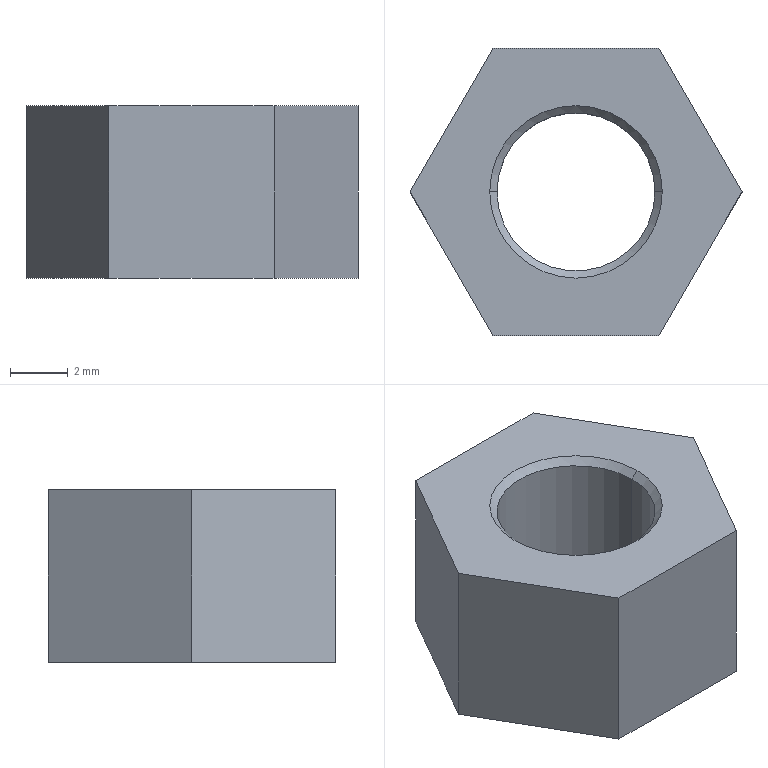Part | STEP file | Tan M6 | 1 solid | 14 faces | box 11.547 x 10 x 6 mm | volume 375.953 mm3 | plane 8 | cone 4 | cylinder 2 | commonest cylinder face diameters 5.5 x2
STEP:
#1=CARTESIAN_POINT('',(0.,0.,0.));
#2=DIRECTION('',(0.,0.,1.));
#3=DIRECTION('',(1.,0.,0.));
#4=AXIS2_PLACEMENT_3D('',#1,#2,#3);
#5=CARTESIAN_POINT('',(-2.75,0.,0.25));
#6=VERTEX_POINT('',#5);
#7=CARTESIAN_POINT('',(-3.,0.,0.));
#8=VERTEX_POINT('',#7);
#9=CARTESIAN_POINT('',(-3.,0.,0.));
#10=DIRECTION('',(-0.7071,0.,-0.7071));
#11=VECTOR('',#10,1.);
#12=LINE('',#9,#11);
#13=CARTESIAN_POINT('',(0.,0.,0.));
#14=DIRECTION('',(0.,0.,-1.));
#15=DIRECTION('',(-1.,0.,0.));
#16=AXIS2_PLACEMENT_3D('',#13,#14,#15);
#17=CONICAL_SURFACE('',#16,3.,0.7854);
#18=CARTESIAN_POINT('',(6.283,0.));
#19=DIRECTION('',(0.,1.));
#20=VECTOR('',#19,1.);
#21=LINE('',#18,#20);
#22=(GEOMETRIC_REPRESENTATION_CONTEXT(2)PARAMETRIC_REPRESENTATION_CONTEXT()REPRESENTATION_CONTEXT('',''));
#23=DEFINITIONAL_REPRESENTATION('',(#21),#22);
#24=PCURVE('',#17,#23);
#25=CARTESIAN_POINT('',(0.,0.,0.));
#26=DIRECTION('',(0.,0.,-1.));
#27=DIRECTION('',(-1.,0.,0.));
#28=AXIS2_PLACEMENT_3D('',#25,#26,#27);
#29=CONICAL_SURFACE('',#28,3.,0.7854);
#30=CARTESIAN_POINT('',(0.,0.));
#31=DIRECTION('',(0.,1.));
#32=VECTOR('',#31,1.);
#33=LINE('',#30,#32);
#34=(GEOMETRIC_REPRESENTATION_CONTEXT(2)PARAMETRIC_REPRESENTATION_CONTEXT()REPRESENTATION_CONTEXT('',''));
#35=DEFINITIONAL_REPRESENTATION('',(#33),#34);
#36=PCURVE('',#29,#35);
#37=SURFACE_CURVE('',#12,(#24,#36),.PCURVE_S1.);
#38=EDGE_CURVE('',#6,#8,#37,.T.);
#39=ORIENTED_EDGE('',*,*,#38,.T.);
#40=CARTESIAN_POINT('',(3.,0.,0.));
#41=VERTEX_POINT('',#40);
#42=CARTESIAN_POINT('',(0.,0.,0.));
#43=DIRECTION('',(0.,0.,1.));
#44=DIRECTION('',(1.,0.,0.));
#45=AXIS2_PLACEMENT_3D('',#42,#43,#44);
#46=CIRCLE('',#45,3.);
#47=CARTESIAN_POINT('',(9.425,0.));
#48=DIRECTION('',(-1.,0.));
#49=VECTOR('',#48,1.);
#50=LINE('',#47,#49);
#51=(GEOMETRIC_REPRESENTATION_CONTEXT(2)PARAMETRIC_REPRESENTATION_CONTEXT()REPRESENTATION_CONTEXT('',''));
#52=DEFINITIONAL_REPRESENTATION('',(#50),#51);
#53=PCURVE('',#17,#52);
#54=CARTESIAN_POINT('',(0.,0.,0.));
#55=DIRECTION('',(0.,0.,1.));
#56=DIRECTION('',(1.,0.,0.));
#57=AXIS2_PLACEMENT_3D('',#54,#55,#56);
#58=PLANE('',#57);
#59=CARTESIAN_POINT('',(0.,0.));
#60=DIRECTION('',(1.,0.));
#61=AXIS2_PLACEMENT_2D('',#59,#60);
#62=CIRCLE('',#61,3.);
#63=(GEOMETRIC_REPRESENTATION_CONTEXT(2)PARAMETRIC_REPRESENTATION_CONTEXT()REPRESENTATION_CONTEXT('',''));
#64=DEFINITIONAL_REPRESENTATION('',(#62),#63);
#65=PCURVE('',#58,#64);
#66=SURFACE_CURVE('',#46,(#53,#65),.PCURVE_S1.);
#67=EDGE_CURVE('',#8,#41,#66,.T.);
#68=ORIENTED_EDGE('',*,*,#67,.T.);
#69=CARTESIAN_POINT('',(2.75,0.,0.25));
#70=VERTEX_POINT('',#69);
#71=CARTESIAN_POINT('',(3.,0.,0.));
#72=DIRECTION('',(0.7071,0.,-0.7071));
#73=VECTOR('',#72,1.);
#74=LINE('',#71,#73);
#75=CARTESIAN_POINT('',(3.142,0.));
#76=DIRECTION('',(0.,1.));
#77=VECTOR('',#76,1.);
#78=LINE('',#75,#77);
#79=(GEOMETRIC_REPRESENTATION_CONTEXT(2)PARAMETRIC_REPRESENTATION_CONTEXT()REPRESENTATION_CONTEXT('',''));
#80=DEFINITIONAL_REPRESENTATION('',(#78),#79);
#81=PCURVE('',#17,#80);
#82=CARTESIAN_POINT('',(3.142,0.));
#83=DIRECTION('',(0.,1.));
#84=VECTOR('',#83,1.);
#85=LINE('',#82,#84);
#86=(GEOMETRIC_REPRESENTATION_CONTEXT(2)PARAMETRIC_REPRESENTATION_CONTEXT()REPRESENTATION_CONTEXT('',''));
#87=DEFINITIONAL_REPRESENTATION('',(#85),#86);
#88=PCURVE('',#29,#87);
#89=SURFACE_CURVE('',#74,(#81,#88),.PCURVE_S1.);
#90=EDGE_CURVE('',#70,#41,#89,.T.);
#91=ORIENTED_EDGE('',*,*,#90,.F.);
#92=CARTESIAN_POINT('',(0.,0.,0.25));
#93=DIRECTION('',(0.,0.,-1.));
#94=DIRECTION('',(1.,0.,0.));
#95=AXIS2_PLACEMENT_3D('',#92,#93,#94);
#96=CIRCLE('',#95,2.75);
#97=CARTESIAN_POINT('',(3.142,-0.25));
#98=DIRECTION('',(1.,0.));
#99=VECTOR('',#98,1.);
#100=LINE('',#97,#99);
#101=(GEOMETRIC_REPRESENTATION_CONTEXT(2)PARAMETRIC_REPRESENTATION_CONTEXT()REPRESENTATION_CONTEXT('',''));
#102=DEFINITIONAL_REPRESENTATION('',(#100),#101);
#103=PCURVE('',#17,#102);
#104=CARTESIAN_POINT('',(0.,0.,6.));
#105=DIRECTION('',(0.,0.,-1.));
#106=DIRECTION('',(-1.,0.,0.));
#107=AXIS2_PLACEMENT_3D('',#104,#105,#106);
#108=CYLINDRICAL_SURFACE('',#107,2.75);
#109=CARTESIAN_POINT('',(3.142,5.75));
#110=DIRECTION('',(1.,0.));
#111=VECTOR('',#110,1.);
#112=LINE('',#109,#111);
#113=(GEOMETRIC_REPRESENTATION_CONTEXT(2)PARAMETRIC_REPRESENTATION_CONTEXT()REPRESENTATION_CONTEXT('',''));
#114=DEFINITIONAL_REPRESENTATION('',(#112),#113);
#115=PCURVE('',#108,#114);
#116=SURFACE_CURVE('',#96,(#103,#115),.PCURVE_S1.);
#117=EDGE_CURVE('',#70,#6,#116,.T.);
#118=ORIENTED_EDGE('',*,*,#117,.T.);
#119=EDGE_LOOP('',(#39,#68,#91,#118));
#120=FACE_BOUND('',#119,.F.);
#121=ADVANCED_FACE('',(#120),#17,.F.);
#122=CARTESIAN_POINT('',(2.75,0.,5.75));
#123=VERTEX_POINT('',#122);
#124=CARTESIAN_POINT('',(3.,0.,6.));
#125=VERTEX_POINT('',#124);
#126=CARTESIAN_POINT('',(2.75,0.,5.75));
#127=DIRECTION('',(0.7071,0.,0.7071));
#128=VECTOR('',#127,1.);
#129=LINE('',#126,#128);
#130=CARTESIAN_POINT('',(0.,0.,5.75));
#131=DIRECTION('',(0.,0.,1.));
#132=DIRECTION('',(1.,0.,0.));
#133=AXIS2_PLACEMENT_3D('',#130,#131,#132);
#134=CONICAL_SURFACE('',#133,2.75,0.7854);
#135=CARTESIAN_POINT('',(6.283,0.));
#136=DIRECTION('',(0.,1.));
#137=VECTOR('',#136,1.);
#138=LINE('',#135,#137);
#139=(GEOMETRIC_REPRESENTATION_CONTEXT(2)PARAMETRIC_REPRESENTATION_CONTEXT()REPRESENTATION_CONTEXT('',''));
#140=DEFINITIONAL_REPRESENTATION('',(#138),#139);
#141=PCURVE('',#134,#140);
#142=CARTESIAN_POINT('',(0.,0.,5.75));
#143=DIRECTION('',(0.,0.,1.));
#144=DIRECTION('',(1.,0.,0.));
#145=AXIS2_PLACEMENT_3D('',#142,#143,#144);
#146=CONICAL_SURFACE('',#145,2.75,0.7854);
#147=CARTESIAN_POINT('',(0.,0.));
#148=DIRECTION('',(0.,1.));
#149=VECTOR('',#148,1.);
#150=LINE('',#147,#149);
#151=(GEOMETRIC_REPRESENTATION_CONTEXT(2)PARAMETRIC_REPRESENTATION_CONTEXT()REPRESENTATION_CONTEXT('',''));
#152=DEFINITIONAL_REPRESENTATION('',(#150),#151);
#153=PCURVE('',#146,#152);
#154=SURFACE_CURVE('',#129,(#141,#153),.PCURVE_S1.);
#155=EDGE_CURVE('',#123,#125,#154,.T.);
#156=ORIENTED_EDGE('',*,*,#155,.T.);
#157=CARTESIAN_POINT('',(-3.,0.,6.));
#158=VERTEX_POINT('',#157);
#159=CARTESIAN_POINT('',(0.,0.,6.));
#160=DIRECTION('',(0.,0.,-1.));
#161=DIRECTION('',(1.,0.,0.));
#162=AXIS2_PLACEMENT_3D('',#159,#160,#161);
#163=CIRCLE('',#162,3.);
#164=CARTESIAN_POINT('',(6.283,0.25));
#165=DIRECTION('',(-1.,0.));
#166=VECTOR('',#165,1.);
#167=LINE('',#164,#166);
#168=(GEOMETRIC_REPRESENTATION_CONTEXT(2)PARAMETRIC_REPRESENTATION_CONTEXT()REPRESENTATION_CONTEXT('',''));
#169=DEFINITIONAL_REPRESENTATION('',(#167),#168);
#170=PCURVE('',#134,#169);
#171=CARTESIAN_POINT('',(0.,0.,6.));
#172=DIRECTION('',(0.,0.,1.));
#173=DIRECTION('',(1.,0.,0.));
#174=AXIS2_PLACEMENT_3D('',#171,#172,#173);
#175=PLANE('',#174);
#176=CARTESIAN_POINT('',(3.,0.));
#177=CARTESIAN_POINT('',(3.,-5.196));
#178=CARTESIAN_POINT('',(-1.5,-2.598));
#179=CARTESIAN_POINT('',(-6.,0.));
#180=CARTESIAN_POINT('',(-1.5,2.598));
#181=CARTESIAN_POINT('',(3.,5.196));
#182=CARTESIAN_POINT('',(3.,0.));
#183=(BOUNDED_CURVE()B_SPLINE_CURVE(2,(#176,#177,#178,#179,#180,#181,#182),.UNSPECIFIED.,.T.,.F.)B_SPLINE_CURVE_WITH_KNOTS((1,2,2,2,2,1),(-2.094,0.,2.094,4.189,6.283,8.378),.UNSPECIFIED.)CURVE()GEOMETRIC_REPRESENTATION_ITEM()RATIONAL_B_SPLINE_CURVE((1.,0.5,1.,0.5,1.,0.5,1.))REPRESENTATION_ITEM(''));
#184=(GEOMETRIC_REPRESENTATION_CONTEXT(2)PARAMETRIC_REPRESENTATION_CONTEXT()REPRESENTATION_CONTEXT('',''));
#185=DEFINITIONAL_REPRESENTATION('',(#183),#184);
#186=PCURVE('',#175,#185);
#187=SURFACE_CURVE('',#163,(#170,#186),.PCURVE_S1.);
#188=EDGE_CURVE('',#125,#158,#187,.T.);
#189=ORIENTED_EDGE('',*,*,#188,.T.);
#190=CARTESIAN_POINT('',(-2.75,0.,5.75));
#191=VERTEX_POINT('',#190);
#192=CARTESIAN_POINT('',(-2.75,0.,5.75));
#193=DIRECTION('',(-0.7071,0.,0.7071));
#194=VECTOR('',#193,1.);
#195=LINE('',#192,#194);
#196=CARTESIAN_POINT('',(3.142,0.));
#197=DIRECTION('',(0.,1.));
#198=VECTOR('',#197,1.);
#199=LINE('',#196,#198);
#200=(GEOMETRIC_REPRESENTATION_CONTEXT(2)PARAMETRIC_REPRESENTATION_CONTEXT()REPRESENTATION_CONTEXT('',''));
#201=DEFINITIONAL_REPRESENTATION('',(#199),#200);
#202=PCURVE('',#134,#201);
#203=CARTESIAN_POINT('',(3.142,0.));
#204=DIRECTION('',(0.,1.));
#205=VECTOR('',#204,1.);
#206=LINE('',#203,#205);
#207=(GEOMETRIC_REPRESENTATION_CONTEXT(2)PARAMETRIC_REPRESENTATION_CONTEXT()REPRESENTATION_CONTEXT('',''));
#208=DEFINITIONAL_REPRESENTATION('',(#206),#207);
#209=PCURVE('',#146,#208);
#210=SURFACE_CURVE('',#195,(#202,#209),.PCURVE_S1.);
#211=EDGE_CURVE('',#191,#158,#210,.T.);
#212=ORIENTED_EDGE('',*,*,#211,.F.);
#213=CARTESIAN_POINT('',(0.,0.,5.75));
#214=DIRECTION('',(0.,0.,1.));
#215=DIRECTION('',(1.,0.,0.));
#216=AXIS2_PLACEMENT_3D('',#213,#214,#215);
#217=CIRCLE('',#216,2.75);
#218=CARTESIAN_POINT('',(0.,0.));
#219=DIRECTION('',(1.,0.));
#220=VECTOR('',#219,1.);
#221=LINE('',#218,#220);
#222=(GEOMETRIC_REPRESENTATION_CONTEXT(2)PARAMETRIC_REPRESENTATION_CONTEXT()REPRESENTATION_CONTEXT('',''));
#223=DEFINITIONAL_REPRESENTATION('',(#221),#222);
#224=PCURVE('',#134,#223);
#225=CARTESIAN_POINT('',(9.425,0.25));
#226=DIRECTION('',(-1.,0.));
#227=VECTOR('',#226,1.);
#228=LINE('',#225,#227);
#229=(GEOMETRIC_REPRESENTATION_CONTEXT(2)PARAMETRIC_REPRESENTATION_CONTEXT()REPRESENTATION_CONTEXT('',''));
#230=DEFINITIONAL_REPRESENTATION('',(#228),#229);
#231=PCURVE('',#108,#230);
#232=SURFACE_CURVE('',#217,(#224,#231),.PCURVE_S1.);
#233=EDGE_CURVE('',#191,#123,#232,.T.);
#234=ORIENTED_EDGE('',*,*,#233,.T.);
#235=EDGE_LOOP('',(#156,#189,#212,#234));
#236=FACE_BOUND('',#235,.F.);
#237=ADVANCED_FACE('',(#236),#134,.F.);
#238=CARTESIAN_POINT('',(-2.75,0.,6.));
#239=DIRECTION('',(0.,0.,-1.));
#240=VECTOR('',#239,1.);
#241=LINE('',#238,#240);
#242=CARTESIAN_POINT('',(6.283,0.));
#243=DIRECTION('',(0.,1.));
#244=VECTOR('',#243,1.);
#245=LINE('',#242,#244);
#246=(GEOMETRIC_REPRESENTATION_CONTEXT(2)PARAMETRIC_REPRESENTATION_CONTEXT()REPRESENTATION_CONTEXT('',''));
#247=DEFINITIONAL_REPRESENTATION('',(#245),#246);
#248=PCURVE('',#108,#247);
#249=CARTESIAN_POINT('',(0.,0.,6.));
#250=DIRECTION('',(0.,0.,-1.));
#251=DIRECTION('',(-1.,0.,0.));
#252=AXIS2_PLACEMENT_3D('',#249,#250,#251);
#253=CYLINDRICAL_SURFACE('',#252,2.75);
#254=CARTESIAN_POINT('',(0.,0.));
#255=DIRECTION('',(0.,1.));
#256=VECTOR('',#255,1.);
#257=LINE('',#254,#256);
#258=(GEOMETRIC_REPRESENTATION_CONTEXT(2)PARAMETRIC_REPRESENTATION_CONTEXT()REPRESENTATION_CONTEXT('',''));
#259=DEFINITIONAL_REPRESENTATION('',(#257),#258);
#260=PCURVE('',#253,#259);
#261=SURFACE_CURVE('',#241,(#248,#260),.PCURVE_S1.);
#262=EDGE_CURVE('',#191,#6,#261,.T.);
#263=ORIENTED_EDGE('',*,*,#262,.T.);
#264=ORIENTED_EDGE('',*,*,#117,.F.);
#265=CARTESIAN_POINT('',(2.75,0.,6.));
#266=DIRECTION('',(0.,0.,-1.));
#267=VECTOR('',#266,1.);
#268=LINE('',#265,#267);
#269=CARTESIAN_POINT('',(3.142,0.));
#270=DIRECTION('',(0.,1.));
#271=VECTOR('',#270,1.);
#272=LINE('',#269,#271);
#273=(GEOMETRIC_REPRESENTATION_CONTEXT(2)PARAMETRIC_REPRESENTATION_CONTEXT()REPRESENTATION_CONTEXT('',''));
#274=DEFINITIONAL_REPRESENTATION('',(#272),#273);
#275=PCURVE('',#108,#274);
#276=CARTESIAN_POINT('',(3.142,0.));
#277=DIRECTION('',(0.,1.));
#278=VECTOR('',#277,1.);
#279=LINE('',#276,#278);
#280=(GEOMETRIC_REPRESENTATION_CONTEXT(2)PARAMETRIC_REPRESENTATION_CONTEXT()REPRESENTATION_CONTEXT('',''));
#281=DEFINITIONAL_REPRESENTATION('',(#279),#280);
#282=PCURVE('',#253,#281);
#283=SURFACE_CURVE('',#268,(#275,#282),.PCURVE_S1.);
#284=EDGE_CURVE('',#123,#70,#283,.T.);
#285=ORIENTED_EDGE('',*,*,#284,.F.);
#286=ORIENTED_EDGE('',*,*,#233,.F.);
#287=EDGE_LOOP('',(#263,#264,#285,#286));
#288=FACE_BOUND('',#287,.F.);
#289=ADVANCED_FACE('',(#288),#108,.F.);
#290=ORIENTED_EDGE('',*,*,#188,.T.);
#291=CARTESIAN_POINT('',(0.,0.,6.));
#292=DIRECTION('',(0.,0.,-1.));
#293=DIRECTION('',(1.,0.,0.));
#294=AXIS2_PLACEMENT_3D('',#291,#292,#293);
#295=CIRCLE('',#294,3.);
#296=CARTESIAN_POINT('',(3.,0.));
#297=CARTESIAN_POINT('',(3.,-5.196));
#298=CARTESIAN_POINT('',(-1.5,-2.598));
#299=CARTESIAN_POINT('',(-6.,0.));
#300=CARTESIAN_POINT('',(-1.5,2.598));
#301=CARTESIAN_POINT('',(3.,5.196));
#302=CARTESIAN_POINT('',(3.,0.));
#303=(BOUNDED_CURVE()B_SPLINE_CURVE(2,(#296,#297,#298,#299,#300,#301,#302),.UNSPECIFIED.,.T.,.F.)B_SPLINE_CURVE_WITH_KNOTS((1,2,2,2,2,1),(-2.094,0.,2.094,4.189,6.283,8.378),.UNSPECIFIED.)CURVE()GEOMETRIC_REPRESENTATION_ITEM()RATIONAL_B_SPLINE_CURVE((1.,0.5,1.,0.5,1.,0.5,1.))REPRESENTATION_ITEM(''));
#304=(GEOMETRIC_REPRESENTATION_CONTEXT(2)PARAMETRIC_REPRESENTATION_CONTEXT()REPRESENTATION_CONTEXT('',''));
#305=DEFINITIONAL_REPRESENTATION('',(#303),#304);
#306=PCURVE('',#175,#305);
#307=CARTESIAN_POINT('',(6.283,0.25));
#308=DIRECTION('',(-1.,0.));
#309=VECTOR('',#308,1.);
#310=LINE('',#307,#309);
#311=(GEOMETRIC_REPRESENTATION_CONTEXT(2)PARAMETRIC_REPRESENTATION_CONTEXT()REPRESENTATION_CONTEXT('',''));
#312=DEFINITIONAL_REPRESENTATION('',(#310),#311);
#313=PCURVE('',#146,#312);
#314=SURFACE_CURVE('',#295,(#306,#313),.PCURVE_S1.);
#315=EDGE_CURVE('',#158,#125,#314,.T.);
#316=ORIENTED_EDGE('',*,*,#315,.T.);
#317=EDGE_LOOP('',(#290,#316));
#318=FACE_BOUND('',#317,.T.);
#319=CARTESIAN_POINT('',(2.887,-5.,6.));
#320=VERTEX_POINT('',#319);
#321=CARTESIAN_POINT('',(5.774,0.,6.));
#322=VERTEX_POINT('',#321);
#323=CARTESIAN_POINT('',(2.887,-5.,6.));
#324=DIRECTION('',(0.5,0.866,0.));
#325=VECTOR('',#324,1.);
#326=LINE('',#323,#325);
#327=CARTESIAN_POINT('',(2.887,-5.));
#328=DIRECTION('',(0.5,0.866));
#329=VECTOR('',#328,1.);
#330=LINE('',#327,#329);
#331=(GEOMETRIC_REPRESENTATION_CONTEXT(2)PARAMETRIC_REPRESENTATION_CONTEXT()REPRESENTATION_CONTEXT('',''));
#332=DEFINITIONAL_REPRESENTATION('',(#330),#331);
#333=PCURVE('',#175,#332);
#334=CARTESIAN_POINT('',(2.887,-5.,6.));
#335=DIRECTION('',(-0.866,0.5,0.));
#336=DIRECTION('',(-0.5,-0.866,0.));
#337=AXIS2_PLACEMENT_3D('',#334,#335,#336);
#338=PLANE('',#337);
#339=CARTESIAN_POINT('',(0.,0.));
#340=DIRECTION('',(-1.,0.));
#341=VECTOR('',#340,1.);
#342=LINE('',#339,#341);
#343=(GEOMETRIC_REPRESENTATION_CONTEXT(2)PARAMETRIC_REPRESENTATION_CONTEXT()REPRESENTATION_CONTEXT('',''));
#344=DEFINITIONAL_REPRESENTATION('',(#342),#343);
#345=PCURVE('',#338,#344);
#346=SURFACE_CURVE('',#326,(#333,#345),.PCURVE_S1.);
#347=EDGE_CURVE('',#320,#322,#346,.T.);
#348=ORIENTED_EDGE('',*,*,#347,.T.);
#349=CARTESIAN_POINT('',(2.887,5.,6.));
#350=VERTEX_POINT('',#349);
#351=CARTESIAN_POINT('',(5.774,0.,6.));
#352=DIRECTION('',(-0.5,0.866,0.));
#353=VECTOR('',#352,1.);
#354=LINE('',#351,#353);
#355=CARTESIAN_POINT('',(5.774,0.));
#356=DIRECTION('',(-0.5,0.866));
#357=VECTOR('',#356,1.);
#358=LINE('',#355,#357);
#359=(GEOMETRIC_REPRESENTATION_CONTEXT(2)PARAMETRIC_REPRESENTATION_CONTEXT()REPRESENTATION_CONTEXT('',''));
#360=DEFINITIONAL_REPRESENTATION('',(#358),#359);
#361=PCURVE('',#175,#360);
#362=CARTESIAN_POINT('',(5.774,0.,6.));
#363=DIRECTION('',(-0.866,-0.5,0.));
#364=DIRECTION('',(0.5,-0.866,0.));
#365=AXIS2_PLACEMENT_3D('',#362,#363,#364);
#366=PLANE('',#365);
#367=CARTESIAN_POINT('',(0.,0.));
#368=DIRECTION('',(-1.,0.));
#369=VECTOR('',#368,1.);
#370=LINE('',#367,#369);
#371=(GEOMETRIC_REPRESENTATION_CONTEXT(2)PARAMETRIC_REPRESENTATION_CONTEXT()REPRESENTATION_CONTEXT('',''));
#372=DEFINITIONAL_REPRESENTATION('',(#370),#371);
#373=PCURVE('',#366,#372);
#374=SURFACE_CURVE('',#354,(#361,#373),.PCURVE_S1.);
#375=EDGE_CURVE('',#322,#350,#374,.T.);
#376=ORIENTED_EDGE('',*,*,#375,.T.);
#377=CARTESIAN_POINT('',(-2.887,5.,6.));
#378=VERTEX_POINT('',#377);
#379=CARTESIAN_POINT('',(2.887,5.,6.));
#380=DIRECTION('',(-1.,0.,0.));
#381=VECTOR('',#380,1.);
#382=LINE('',#379,#381);
#383=CARTESIAN_POINT('',(2.887,5.));
#384=DIRECTION('',(-1.,0.));
#385=VECTOR('',#384,1.);
#386=LINE('',#383,#385);
#387=(GEOMETRIC_REPRESENTATION_CONTEXT(2)PARAMETRIC_REPRESENTATION_CONTEXT()REPRESENTATION_CONTEXT('',''));
#388=DEFINITIONAL_REPRESENTATION('',(#386),#387);
#389=PCURVE('',#175,#388);
#390=CARTESIAN_POINT('',(2.887,5.,6.));
#391=DIRECTION('',(0.,-1.,0.));
#392=DIRECTION('',(0.,0.,-1.));
#393=AXIS2_PLACEMENT_3D('',#390,#391,#392);
#394=PLANE('',#393);
#395=CARTESIAN_POINT('',(0.,0.));
#396=DIRECTION('',(0.,-1.));
#397=VECTOR('',#396,1.);
#398=LINE('',#395,#397);
#399=(GEOMETRIC_REPRESENTATION_CONTEXT(2)PARAMETRIC_REPRESENTATION_CONTEXT()REPRESENTATION_CONTEXT('',''));
#400=DEFINITIONAL_REPRESENTATION('',(#398),#399);
#401=PCURVE('',#394,#400);
#402=SURFACE_CURVE('',#382,(#389,#401),.PCURVE_S1.);
#403=EDGE_CURVE('',#350,#378,#402,.T.);
#404=ORIENTED_EDGE('',*,*,#403,.T.);
#405=CARTESIAN_POINT('',(-5.774,0.,6.));
#406=VERTEX_POINT('',#405);
#407=CARTESIAN_POINT('',(-2.887,5.,6.));
#408=DIRECTION('',(-0.5,-0.866,0.));
#409=VECTOR('',#408,1.);
#410=LINE('',#407,#409);
#411=CARTESIAN_POINT('',(-2.887,5.));
#412=DIRECTION('',(-0.5,-0.866));
#413=VECTOR('',#412,1.);
#414=LINE('',#411,#413);
#415=(GEOMETRIC_REPRESENTATION_CONTEXT(2)PARAMETRIC_REPRESENTATION_CONTEXT()REPRESENTATION_CONTEXT('',''));
#416=DEFINITIONAL_REPRESENTATION('',(#414),#415);
#417=PCURVE('',#175,#416);
#418=CARTESIAN_POINT('',(-2.887,5.,6.));
#419=DIRECTION('',(0.866,-0.5,0.));
#420=DIRECTION('',(0.5,0.866,0.));
#421=AXIS2_PLACEMENT_3D('',#418,#419,#420);
#422=PLANE('',#421);
#423=CARTESIAN_POINT('',(0.,0.));
#424=DIRECTION('',(-1.,0.));
#425=VECTOR('',#424,1.);
#426=LINE('',#423,#425);
#427=(GEOMETRIC_REPRESENTATION_CONTEXT(2)PARAMETRIC_REPRESENTATION_CONTEXT()REPRESENTATION_CONTEXT('',''));
#428=DEFINITIONAL_REPRESENTATION('',(#426),#427);
#429=PCURVE('',#422,#428);
#430=SURFACE_CURVE('',#410,(#417,#429),.PCURVE_S1.);
#431=EDGE_CURVE('',#378,#406,#430,.T.);
#432=ORIENTED_EDGE('',*,*,#431,.T.);
#433=CARTESIAN_POINT('',(-2.887,-5.,6.));
#434=VERTEX_POINT('',#433);
#435=CARTESIAN_POINT('',(-5.774,0.,6.));
#436=DIRECTION('',(0.5,-0.866,0.));
#437=VECTOR('',#436,1.);
#438=LINE('',#435,#437);
#439=CARTESIAN_POINT('',(-5.774,0.));
#440=DIRECTION('',(0.5,-0.866));
#441=VECTOR('',#440,1.);
#442=LINE('',#439,#441);
#443=(GEOMETRIC_REPRESENTATION_CONTEXT(2)PARAMETRIC_REPRESENTATION_CONTEXT()REPRESENTATION_CONTEXT('',''));
#444=DEFINITIONAL_REPRESENTATION('',(#442),#443);
#445=PCURVE('',#175,#444);
#446=CARTESIAN_POINT('',(-5.774,0.,6.));
#447=DIRECTION('',(0.866,0.5,0.));
#448=DIRECTION('',(-0.5,0.866,0.));
#449=AXIS2_PLACEMENT_3D('',#446,#447,#448);
#450=PLANE('',#449);
#451=CARTESIAN_POINT('',(0.,0.));
#452=DIRECTION('',(-1.,0.));
#453=VECTOR('',#452,1.);
#454=LINE('',#451,#453);
#455=(GEOMETRIC_REPRESENTATION_CONTEXT(2)PARAMETRIC_REPRESENTATION_CONTEXT()REPRESENTATION_CONTEXT('',''));
#456=DEFINITIONAL_REPRESENTATION('',(#454),#455);
#457=PCURVE('',#450,#456);
#458=SURFACE_CURVE('',#438,(#445,#457),.PCURVE_S1.);
#459=EDGE_CURVE('',#406,#434,#458,.T.);
#460=ORIENTED_EDGE('',*,*,#459,.T.);
#461=CARTESIAN_POINT('',(-2.887,-5.,6.));
#462=DIRECTION('',(1.,0.,0.));
#463=VECTOR('',#462,1.);
#464=LINE('',#461,#463);
#465=CARTESIAN_POINT('',(-2.887,-5.));
#466=DIRECTION('',(1.,0.));
#467=VECTOR('',#466,1.);
#468=LINE('',#465,#467);
#469=(GEOMETRIC_REPRESENTATION_CONTEXT(2)PARAMETRIC_REPRESENTATION_CONTEXT()REPRESENTATION_CONTEXT('',''));
#470=DEFINITIONAL_REPRESENTATION('',(#468),#469);
#471=PCURVE('',#175,#470);
#472=CARTESIAN_POINT('',(-2.887,-5.,6.));
#473=DIRECTION('',(0.,1.,0.));
#474=DIRECTION('',(-1.,0.,0.));
#475=AXIS2_PLACEMENT_3D('',#472,#473,#474);
#476=PLANE('',#475);
#477=CARTESIAN_POINT('',(0.,0.));
#478=DIRECTION('',(-1.,0.));
#479=VECTOR('',#478,1.);
#480=LINE('',#477,#479);
#481=(GEOMETRIC_REPRESENTATION_CONTEXT(2)PARAMETRIC_REPRESENTATION_CONTEXT()REPRESENTATION_CONTEXT('',''));
#482=DEFINITIONAL_REPRESENTATION('',(#480),#481);
#483=PCURVE('',#476,#482);
#484=SURFACE_CURVE('',#464,(#471,#483),.PCURVE_S1.);
#485=EDGE_CURVE('',#434,#320,#484,.T.);
#486=ORIENTED_EDGE('',*,*,#485,.T.);
#487=EDGE_LOOP('',(#348,#376,#404,#432,#460,#486));
#488=FACE_BOUND('',#487,.T.);
#489=ADVANCED_FACE('',(#318,#488),#175,.T.);
#490=ORIENTED_EDGE('',*,*,#67,.T.);
#491=CARTESIAN_POINT('',(0.,0.,0.));
#492=DIRECTION('',(0.,0.,1.));
#493=DIRECTION('',(1.,0.,0.));
#494=AXIS2_PLACEMENT_3D('',#491,#492,#493);
#495=CIRCLE('',#494,3.);
#496=CARTESIAN_POINT('',(0.,0.));
#497=DIRECTION('',(1.,0.));
#498=AXIS2_PLACEMENT_2D('',#496,#497);
#499=CIRCLE('',#498,3.);
#500=(GEOMETRIC_REPRESENTATION_CONTEXT(2)PARAMETRIC_REPRESENTATION_CONTEXT()REPRESENTATION_CONTEXT('',''));
#501=DEFINITIONAL_REPRESENTATION('',(#499),#500);
#502=PCURVE('',#58,#501);
#503=CARTESIAN_POINT('',(3.142,0.));
#504=DIRECTION('',(-1.,0.));
#505=VECTOR('',#504,1.);
#506=LINE('',#503,#505);
#507=(GEOMETRIC_REPRESENTATION_CONTEXT(2)PARAMETRIC_REPRESENTATION_CONTEXT()REPRESENTATION_CONTEXT('',''));
#508=DEFINITIONAL_REPRESENTATION('',(#506),#507);
#509=PCURVE('',#29,#508);
#510=SURFACE_CURVE('',#495,(#502,#509),.PCURVE_S1.);
#511=EDGE_CURVE('',#41,#8,#510,.T.);
#512=ORIENTED_EDGE('',*,*,#511,.T.);
#513=EDGE_LOOP('',(#490,#512));
#514=FACE_BOUND('',#513,.T.);
#515=CARTESIAN_POINT('',(2.887,-5.,0.));
#516=VERTEX_POINT('',#515);
#517=CARTESIAN_POINT('',(5.774,0.,0.));
#518=VERTEX_POINT('',#517);
#519=CARTESIAN_POINT('',(2.887,-5.,0.));
#520=DIRECTION('',(0.5,0.866,0.));
#521=VECTOR('',#520,1.);
#522=LINE('',#519,#521);
#523=CARTESIAN_POINT('',(2.887,-5.));
#524=DIRECTION('',(0.5,0.866));
#525=VECTOR('',#524,1.);
#526=LINE('',#523,#525);
#527=(GEOMETRIC_REPRESENTATION_CONTEXT(2)PARAMETRIC_REPRESENTATION_CONTEXT()REPRESENTATION_CONTEXT('',''));
#528=DEFINITIONAL_REPRESENTATION('',(#526),#527);
#529=PCURVE('',#58,#528);
#530=CARTESIAN_POINT('',(0.,-6.));
#531=DIRECTION('',(-1.,0.));
#532=VECTOR('',#531,1.);
#533=LINE('',#530,#532);
#534=(GEOMETRIC_REPRESENTATION_CONTEXT(2)PARAMETRIC_REPRESENTATION_CONTEXT()REPRESENTATION_CONTEXT('',''));
#535=DEFINITIONAL_REPRESENTATION('',(#533),#534);
#536=PCURVE('',#338,#535);
#537=SURFACE_CURVE('',#522,(#529,#536),.PCURVE_S1.);
#538=EDGE_CURVE('',#516,#518,#537,.T.);
#539=ORIENTED_EDGE('',*,*,#538,.F.);
#540=CARTESIAN_POINT('',(-2.887,-5.,0.));
#541=VERTEX_POINT('',#540);
#542=CARTESIAN_POINT('',(-2.887,-5.,0.));
#543=DIRECTION('',(1.,0.,0.));
#544=VECTOR('',#543,1.);
#545=LINE('',#542,#544);
#546=CARTESIAN_POINT('',(-2.887,-5.));
#547=DIRECTION('',(1.,0.));
#548=VECTOR('',#547,1.);
#549=LINE('',#546,#548);
#550=(GEOMETRIC_REPRESENTATION_CONTEXT(2)PARAMETRIC_REPRESENTATION_CONTEXT()REPRESENTATION_CONTEXT('',''));
#551=DEFINITIONAL_REPRESENTATION('',(#549),#550);
#552=PCURVE('',#58,#551);
#553=CARTESIAN_POINT('',(0.,-6.));
#554=DIRECTION('',(-1.,0.));
#555=VECTOR('',#554,1.);
#556=LINE('',#553,#555);
#557=(GEOMETRIC_REPRESENTATION_CONTEXT(2)PARAMETRIC_REPRESENTATION_CONTEXT()REPRESENTATION_CONTEXT('',''));
#558=DEFINITIONAL_REPRESENTATION('',(#556),#557);
#559=PCURVE('',#476,#558);
#560=SURFACE_CURVE('',#545,(#552,#559),.PCURVE_S1.);
#561=EDGE_CURVE('',#541,#516,#560,.T.);
#562=ORIENTED_EDGE('',*,*,#561,.F.);
#563=CARTESIAN_POINT('',(-5.774,0.,0.));
#564=VERTEX_POINT('',#563);
#565=CARTESIAN_POINT('',(-5.774,0.,0.));
#566=DIRECTION('',(0.5,-0.866,0.));
#567=VECTOR('',#566,1.);
#568=LINE('',#565,#567);
#569=CARTESIAN_POINT('',(-5.774,0.));
#570=DIRECTION('',(0.5,-0.866));
#571=VECTOR('',#570,1.);
#572=LINE('',#569,#571);
#573=(GEOMETRIC_REPRESENTATION_CONTEXT(2)PARAMETRIC_REPRESENTATION_CONTEXT()REPRESENTATION_CONTEXT('',''));
#574=DEFINITIONAL_REPRESENTATION('',(#572),#573);
#575=PCURVE('',#58,#574);
#576=CARTESIAN_POINT('',(0.,-6.));
#577=DIRECTION('',(-1.,0.));
#578=VECTOR('',#577,1.);
#579=LINE('',#576,#578);
#580=(GEOMETRIC_REPRESENTATION_CONTEXT(2)PARAMETRIC_REPRESENTATION_CONTEXT()REPRESENTATION_CONTEXT('',''));
#581=DEFINITIONAL_REPRESENTATION('',(#579),#580);
#582=PCURVE('',#450,#581);
#583=SURFACE_CURVE('',#568,(#575,#582),.PCURVE_S1.);
#584=EDGE_CURVE('',#564,#541,#583,.T.);
#585=ORIENTED_EDGE('',*,*,#584,.F.);
#586=CARTESIAN_POINT('',(-2.887,5.,0.));
#587=VERTEX_POINT('',#586);
#588=CARTESIAN_POINT('',(-2.887,5.,0.));
#589=DIRECTION('',(-0.5,-0.866,0.));
#590=VECTOR('',#589,1.);
#591=LINE('',#588,#590);
#592=CARTESIAN_POINT('',(-2.887,5.));
#593=DIRECTION('',(-0.5,-0.866));
#594=VECTOR('',#593,1.);
#595=LINE('',#592,#594);
#596=(GEOMETRIC_REPRESENTATION_CONTEXT(2)PARAMETRIC_REPRESENTATION_CONTEXT()REPRESENTATION_CONTEXT('',''));
#597=DEFINITIONAL_REPRESENTATION('',(#595),#596);
#598=PCURVE('',#58,#597);
#599=CARTESIAN_POINT('',(0.,-6.));
#600=DIRECTION('',(-1.,0.));
#601=VECTOR('',#600,1.);
#602=LINE('',#599,#601);
#603=(GEOMETRIC_REPRESENTATION_CONTEXT(2)PARAMETRIC_REPRESENTATION_CONTEXT()REPRESENTATION_CONTEXT('',''));
#604=DEFINITIONAL_REPRESENTATION('',(#602),#603);
#605=PCURVE('',#422,#604);
#606=SURFACE_CURVE('',#591,(#598,#605),.PCURVE_S1.);
#607=EDGE_CURVE('',#587,#564,#606,.T.);
#608=ORIENTED_EDGE('',*,*,#607,.F.);
#609=CARTESIAN_POINT('',(2.887,5.,0.));
#610=VERTEX_POINT('',#609);
#611=CARTESIAN_POINT('',(2.887,5.,0.));
#612=DIRECTION('',(-1.,0.,0.));
#613=VECTOR('',#612,1.);
#614=LINE('',#611,#613);
#615=CARTESIAN_POINT('',(2.887,5.));
#616=DIRECTION('',(-1.,0.));
#617=VECTOR('',#616,1.);
#618=LINE('',#615,#617);
#619=(GEOMETRIC_REPRESENTATION_CONTEXT(2)PARAMETRIC_REPRESENTATION_CONTEXT()REPRESENTATION_CONTEXT('',''));
#620=DEFINITIONAL_REPRESENTATION('',(#618),#619);
#621=PCURVE('',#58,#620);
#622=CARTESIAN_POINT('',(6.,0.));
#623=DIRECTION('',(0.,-1.));
#624=VECTOR('',#623,1.);
#625=LINE('',#622,#624);
#626=(GEOMETRIC_REPRESENTATION_CONTEXT(2)PARAMETRIC_REPRESENTATION_CONTEXT()REPRESENTATION_CONTEXT('',''));
#627=DEFINITIONAL_REPRESENTATION('',(#625),#626);
#628=PCURVE('',#394,#627);
#629=SURFACE_CURVE('',#614,(#621,#628),.PCURVE_S1.);
#630=EDGE_CURVE('',#610,#587,#629,.T.);
#631=ORIENTED_EDGE('',*,*,#630,.F.);
#632=CARTESIAN_POINT('',(5.774,0.,0.));
#633=DIRECTION('',(-0.5,0.866,0.));
#634=VECTOR('',#633,1.);
#635=LINE('',#632,#634);
#636=CARTESIAN_POINT('',(5.774,0.));
#637=DIRECTION('',(-0.5,0.866));
#638=VECTOR('',#637,1.);
#639=LINE('',#636,#638);
#640=(GEOMETRIC_REPRESENTATION_CONTEXT(2)PARAMETRIC_REPRESENTATION_CONTEXT()REPRESENTATION_CONTEXT('',''));
#641=DEFINITIONAL_REPRESENTATION('',(#639),#640);
#642=PCURVE('',#58,#641);
#643=CARTESIAN_POINT('',(0.,-6.));
#644=DIRECTION('',(-1.,0.));
#645=VECTOR('',#644,1.);
#646=LINE('',#643,#645);
#647=(GEOMETRIC_REPRESENTATION_CONTEXT(2)PARAMETRIC_REPRESENTATION_CONTEXT()REPRESENTATION_CONTEXT('',''));
#648=DEFINITIONAL_REPRESENTATION('',(#646),#647);
#649=PCURVE('',#366,#648);
#650=SURFACE_CURVE('',#635,(#642,#649),.PCURVE_S1.);
#651=EDGE_CURVE('',#518,#610,#650,.T.);
#652=ORIENTED_EDGE('',*,*,#651,.F.);
#653=EDGE_LOOP('',(#539,#562,#585,#608,#631,#652));
#654=FACE_BOUND('',#653,.T.);
#655=ADVANCED_FACE('',(#514,#654),#58,.F.);
#656=ORIENTED_EDGE('',*,*,#538,.T.);
#657=CARTESIAN_POINT('',(5.774,0.,6.));
#658=DIRECTION('',(0.,0.,-1.));
#659=VECTOR('',#658,1.);
#660=LINE('',#657,#659);
#661=CARTESIAN_POINT('',(-5.774,0.));
#662=DIRECTION('',(0.,-1.));
#663=VECTOR('',#662,1.);
#664=LINE('',#661,#663);
#665=(GEOMETRIC_REPRESENTATION_CONTEXT(2)PARAMETRIC_REPRESENTATION_CONTEXT()REPRESENTATION_CONTEXT('',''));
#666=DEFINITIONAL_REPRESENTATION('',(#664),#665);
#667=PCURVE('',#338,#666);
#668=CARTESIAN_POINT('',(0.,0.));
#669=DIRECTION('',(0.,-1.));
#670=VECTOR('',#669,1.);
#671=LINE('',#668,#670);
#672=(GEOMETRIC_REPRESENTATION_CONTEXT(2)PARAMETRIC_REPRESENTATION_CONTEXT()REPRESENTATION_CONTEXT('',''));
#673=DEFINITIONAL_REPRESENTATION('',(#671),#672);
#674=PCURVE('',#366,#673);
#675=SURFACE_CURVE('',#660,(#667,#674),.PCURVE_S1.);
#676=EDGE_CURVE('',#322,#518,#675,.T.);
#677=ORIENTED_EDGE('',*,*,#676,.F.);
#678=ORIENTED_EDGE('',*,*,#347,.F.);
#679=CARTESIAN_POINT('',(2.887,-5.,6.));
#680=DIRECTION('',(0.,0.,-1.));
#681=VECTOR('',#680,1.);
#682=LINE('',#679,#681);
#683=CARTESIAN_POINT('',(0.,0.));
#684=DIRECTION('',(0.,-1.));
#685=VECTOR('',#684,1.);
#686=LINE('',#683,#685);
#687=(GEOMETRIC_REPRESENTATION_CONTEXT(2)PARAMETRIC_REPRESENTATION_CONTEXT()REPRESENTATION_CONTEXT('',''));
#688=DEFINITIONAL_REPRESENTATION('',(#686),#687);
#689=PCURVE('',#338,#688);
#690=CARTESIAN_POINT('',(-5.774,0.));
#691=DIRECTION('',(0.,-1.));
#692=VECTOR('',#691,1.);
#693=LINE('',#690,#692);
#694=(GEOMETRIC_REPRESENTATION_CONTEXT(2)PARAMETRIC_REPRESENTATION_CONTEXT()REPRESENTATION_CONTEXT('',''));
#695=DEFINITIONAL_REPRESENTATION('',(#693),#694);
#696=PCURVE('',#476,#695);
#697=SURFACE_CURVE('',#682,(#689,#696),.PCURVE_S1.);
#698=EDGE_CURVE('',#320,#516,#697,.T.);
#699=ORIENTED_EDGE('',*,*,#698,.T.);
#700=EDGE_LOOP('',(#656,#677,#678,#699));
#701=FACE_BOUND('',#700,.T.);
#702=ADVANCED_FACE('',(#701),#338,.F.);
#703=ORIENTED_EDGE('',*,*,#651,.T.);
#704=CARTESIAN_POINT('',(2.887,5.,6.));
#705=DIRECTION('',(0.,0.,-1.));
#706=VECTOR('',#705,1.);
#707=LINE('',#704,#706);
#708=CARTESIAN_POINT('',(-5.774,0.));
#709=DIRECTION('',(0.,-1.));
#710=VECTOR('',#709,1.);
#711=LINE('',#708,#710);
#712=(GEOMETRIC_REPRESENTATION_CONTEXT(2)PARAMETRIC_REPRESENTATION_CONTEXT()REPRESENTATION_CONTEXT('',''));
#713=DEFINITIONAL_REPRESENTATION('',(#711),#712);
#714=PCURVE('',#366,#713);
#715=CARTESIAN_POINT('',(0.,0.));
#716=DIRECTION('',(1.,0.));
#717=VECTOR('',#716,1.);
#718=LINE('',#715,#717);
#719=(GEOMETRIC_REPRESENTATION_CONTEXT(2)PARAMETRIC_REPRESENTATION_CONTEXT()REPRESENTATION_CONTEXT('',''));
#720=DEFINITIONAL_REPRESENTATION('',(#718),#719);
#721=PCURVE('',#394,#720);
#722=SURFACE_CURVE('',#707,(#714,#721),.PCURVE_S1.);
#723=EDGE_CURVE('',#350,#610,#722,.T.);
#724=ORIENTED_EDGE('',*,*,#723,.F.);
#725=ORIENTED_EDGE('',*,*,#375,.F.);
#726=ORIENTED_EDGE('',*,*,#676,.T.);
#727=EDGE_LOOP('',(#703,#724,#725,#726));
#728=FACE_BOUND('',#727,.T.);
#729=ADVANCED_FACE('',(#728),#366,.F.);
#730=ORIENTED_EDGE('',*,*,#630,.T.);
#731=CARTESIAN_POINT('',(-2.887,5.,6.));
#732=DIRECTION('',(0.,0.,-1.));
#733=VECTOR('',#732,1.);
#734=LINE('',#731,#733);
#735=CARTESIAN_POINT('',(0.,-5.774));
#736=DIRECTION('',(1.,0.));
#737=VECTOR('',#736,1.);
#738=LINE('',#735,#737);
#739=(GEOMETRIC_REPRESENTATION_CONTEXT(2)PARAMETRIC_REPRESENTATION_CONTEXT()REPRESENTATION_CONTEXT('',''));
#740=DEFINITIONAL_REPRESENTATION('',(#738),#739);
#741=PCURVE('',#394,#740);
#742=CARTESIAN_POINT('',(0.,0.));
#743=DIRECTION('',(0.,-1.));
#744=VECTOR('',#743,1.);
#745=LINE('',#742,#744);
#746=(GEOMETRIC_REPRESENTATION_CONTEXT(2)PARAMETRIC_REPRESENTATION_CONTEXT()REPRESENTATION_CONTEXT('',''));
#747=DEFINITIONAL_REPRESENTATION('',(#745),#746);
#748=PCURVE('',#422,#747);
#749=SURFACE_CURVE('',#734,(#741,#748),.PCURVE_S1.);
#750=EDGE_CURVE('',#378,#587,#749,.T.);
#751=ORIENTED_EDGE('',*,*,#750,.F.);
#752=ORIENTED_EDGE('',*,*,#403,.F.);
#753=ORIENTED_EDGE('',*,*,#723,.T.);
#754=EDGE_LOOP('',(#730,#751,#752,#753));
#755=FACE_BOUND('',#754,.T.);
#756=ADVANCED_FACE('',(#755),#394,.F.);
#757=ORIENTED_EDGE('',*,*,#607,.T.);
#758=CARTESIAN_POINT('',(-5.774,0.,6.));
#759=DIRECTION('',(0.,0.,-1.));
#760=VECTOR('',#759,1.);
#761=LINE('',#758,#760);
#762=CARTESIAN_POINT('',(-5.774,0.));
#763=DIRECTION('',(0.,-1.));
#764=VECTOR('',#763,1.);
#765=LINE('',#762,#764);
#766=(GEOMETRIC_REPRESENTATION_CONTEXT(2)PARAMETRIC_REPRESENTATION_CONTEXT()REPRESENTATION_CONTEXT('',''));
#767=DEFINITIONAL_REPRESENTATION('',(#765),#766);
#768=PCURVE('',#422,#767);
#769=CARTESIAN_POINT('',(0.,0.));
#770=DIRECTION('',(0.,-1.));
#771=VECTOR('',#770,1.);
#772=LINE('',#769,#771);
#773=(GEOMETRIC_REPRESENTATION_CONTEXT(2)PARAMETRIC_REPRESENTATION_CONTEXT()REPRESENTATION_CONTEXT('',''));
#774=DEFINITIONAL_REPRESENTATION('',(#772),#773);
#775=PCURVE('',#450,#774);
#776=SURFACE_CURVE('',#761,(#768,#775),.PCURVE_S1.);
#777=EDGE_CURVE('',#406,#564,#776,.T.);
#778=ORIENTED_EDGE('',*,*,#777,.F.);
#779=ORIENTED_EDGE('',*,*,#431,.F.);
#780=ORIENTED_EDGE('',*,*,#750,.T.);
#781=EDGE_LOOP('',(#757,#778,#779,#780));
#782=FACE_BOUND('',#781,.T.);
#783=ADVANCED_FACE('',(#782),#422,.F.);
#784=ORIENTED_EDGE('',*,*,#584,.T.);
#785=CARTESIAN_POINT('',(-2.887,-5.,6.));
#786=DIRECTION('',(0.,0.,-1.));
#787=VECTOR('',#786,1.);
#788=LINE('',#785,#787);
#789=CARTESIAN_POINT('',(-5.774,0.));
#790=DIRECTION('',(0.,-1.));
#791=VECTOR('',#790,1.);
#792=LINE('',#789,#791);
#793=(GEOMETRIC_REPRESENTATION_CONTEXT(2)PARAMETRIC_REPRESENTATION_CONTEXT()REPRESENTATION_CONTEXT('',''));
#794=DEFINITIONAL_REPRESENTATION('',(#792),#793);
#795=PCURVE('',#450,#794);
#796=CARTESIAN_POINT('',(0.,0.));
#797=DIRECTION('',(0.,-1.));
#798=VECTOR('',#797,1.);
#799=LINE('',#796,#798);
#800=(GEOMETRIC_REPRESENTATION_CONTEXT(2)PARAMETRIC_REPRESENTATION_CONTEXT()REPRESENTATION_CONTEXT('',''));
#801=DEFINITIONAL_REPRESENTATION('',(#799),#800);
#802=PCURVE('',#476,#801);
#803=SURFACE_CURVE('',#788,(#795,#802),.PCURVE_S1.);
#804=EDGE_CURVE('',#434,#541,#803,.T.);
#805=ORIENTED_EDGE('',*,*,#804,.F.);
#806=ORIENTED_EDGE('',*,*,#459,.F.);
#807=ORIENTED_EDGE('',*,*,#777,.T.);
#808=EDGE_LOOP('',(#784,#805,#806,#807));
#809=FACE_BOUND('',#808,.T.);
#810=ADVANCED_FACE('',(#809),#450,.F.);
#811=ORIENTED_EDGE('',*,*,#561,.T.);
#812=ORIENTED_EDGE('',*,*,#698,.F.);
#813=ORIENTED_EDGE('',*,*,#485,.F.);
#814=ORIENTED_EDGE('',*,*,#804,.T.);
#815=EDGE_LOOP('',(#811,#812,#813,#814));
#816=FACE_BOUND('',#815,.T.);
#817=ADVANCED_FACE('',(#816),#476,.F.);
#818=CARTESIAN_POINT('',(0.,0.,0.25));
#819=DIRECTION('',(0.,0.,-1.));
#820=DIRECTION('',(1.,0.,0.));
#821=AXIS2_PLACEMENT_3D('',#818,#819,#820);
#822=CIRCLE('',#821,2.75);
#823=CARTESIAN_POINT('',(-3.142,5.75));
#824=DIRECTION('',(1.,0.));
#825=VECTOR('',#824,1.);
#826=LINE('',#823,#825);
#827=(GEOMETRIC_REPRESENTATION_CONTEXT(2)PARAMETRIC_REPRESENTATION_CONTEXT()REPRESENTATION_CONTEXT('',''));
#828=DEFINITIONAL_REPRESENTATION('',(#826),#827);
#829=PCURVE('',#253,#828);
#830=CARTESIAN_POINT('',(-3.142,-0.25));
#831=DIRECTION('',(1.,0.));
#832=VECTOR('',#831,1.);
#833=LINE('',#830,#832);
#834=(GEOMETRIC_REPRESENTATION_CONTEXT(2)PARAMETRIC_REPRESENTATION_CONTEXT()REPRESENTATION_CONTEXT('',''));
#835=DEFINITIONAL_REPRESENTATION('',(#833),#834);
#836=PCURVE('',#29,#835);
#837=SURFACE_CURVE('',#822,(#829,#836),.PCURVE_S1.);
#838=EDGE_CURVE('',#6,#70,#837,.T.);
#839=ORIENTED_EDGE('',*,*,#838,.F.);
#840=ORIENTED_EDGE('',*,*,#262,.F.);
#841=CARTESIAN_POINT('',(0.,0.,5.75));
#842=DIRECTION('',(0.,0.,1.));
#843=DIRECTION('',(1.,0.,0.));
#844=AXIS2_PLACEMENT_3D('',#841,#842,#843);
#845=CIRCLE('',#844,2.75);
#846=CARTESIAN_POINT('',(3.142,0.25));
#847=DIRECTION('',(-1.,0.));
#848=VECTOR('',#847,1.);
#849=LINE('',#846,#848);
#850=(GEOMETRIC_REPRESENTATION_CONTEXT(2)PARAMETRIC_REPRESENTATION_CONTEXT()REPRESENTATION_CONTEXT('',''));
#851=DEFINITIONAL_REPRESENTATION('',(#849),#850);
#852=PCURVE('',#253,#851);
#853=CARTESIAN_POINT('',(0.,0.));
#854=DIRECTION('',(1.,0.));
#855=VECTOR('',#854,1.);
#856=LINE('',#853,#855);
#857=(GEOMETRIC_REPRESENTATION_CONTEXT(2)PARAMETRIC_REPRESENTATION_CONTEXT()REPRESENTATION_CONTEXT('',''));
#858=DEFINITIONAL_REPRESENTATION('',(#856),#857);
#859=PCURVE('',#146,#858);
#860=SURFACE_CURVE('',#845,(#852,#859),.PCURVE_S1.);
#861=EDGE_CURVE('',#123,#191,#860,.T.);
#862=ORIENTED_EDGE('',*,*,#861,.F.);
#863=ORIENTED_EDGE('',*,*,#284,.T.);
#864=EDGE_LOOP('',(#839,#840,#862,#863));
#865=FACE_BOUND('',#864,.F.);
#866=ADVANCED_FACE('',(#865),#253,.F.);
#867=ORIENTED_EDGE('',*,*,#315,.T.);
#868=ORIENTED_EDGE('',*,*,#155,.F.);
#869=ORIENTED_EDGE('',*,*,#861,.T.);
#870=ORIENTED_EDGE('',*,*,#211,.T.);
#871=EDGE_LOOP('',(#867,#868,#869,#870));
#872=FACE_BOUND('',#871,.F.);
#873=ADVANCED_FACE('',(#872),#146,.F.);
#874=ORIENTED_EDGE('',*,*,#511,.T.);
#875=ORIENTED_EDGE('',*,*,#38,.F.);
#876=ORIENTED_EDGE('',*,*,#838,.T.);
#877=ORIENTED_EDGE('',*,*,#90,.T.);
#878=EDGE_LOOP('',(#874,#875,#876,#877));
#879=FACE_BOUND('',#878,.F.);
#880=ADVANCED_FACE('',(#879),#29,.F.);
#881=CLOSED_SHELL('',(#121,#237,#289,#489,#655,#702,#729,#756,#783,#810,#817,#866,#873,#880));
#882=MANIFOLD_SOLID_BREP('',#881);
#883=(LENGTH_UNIT()NAMED_UNIT(*)SI_UNIT(.MILLI.,.METRE.));
#884=UNCERTAINTY_MEASURE_WITH_UNIT(LENGTH_MEASURE(0.0000001),#883,'','');
#885=(NAMED_UNIT(*)PLANE_ANGLE_UNIT()SI_UNIT($,.RADIAN.));
#886=(NAMED_UNIT(*)SI_UNIT($,.STERADIAN.)SOLID_ANGLE_UNIT());
#887=(GEOMETRIC_REPRESENTATION_CONTEXT(3)GLOBAL_UNCERTAINTY_ASSIGNED_CONTEXT((#884))GLOBAL_UNIT_ASSIGNED_CONTEXT((#883,#885,#886))REPRESENTATION_CONTEXT('',''));
#888=ADVANCED_BREP_SHAPE_REPRESENTATION('',(#4,#882),#887);